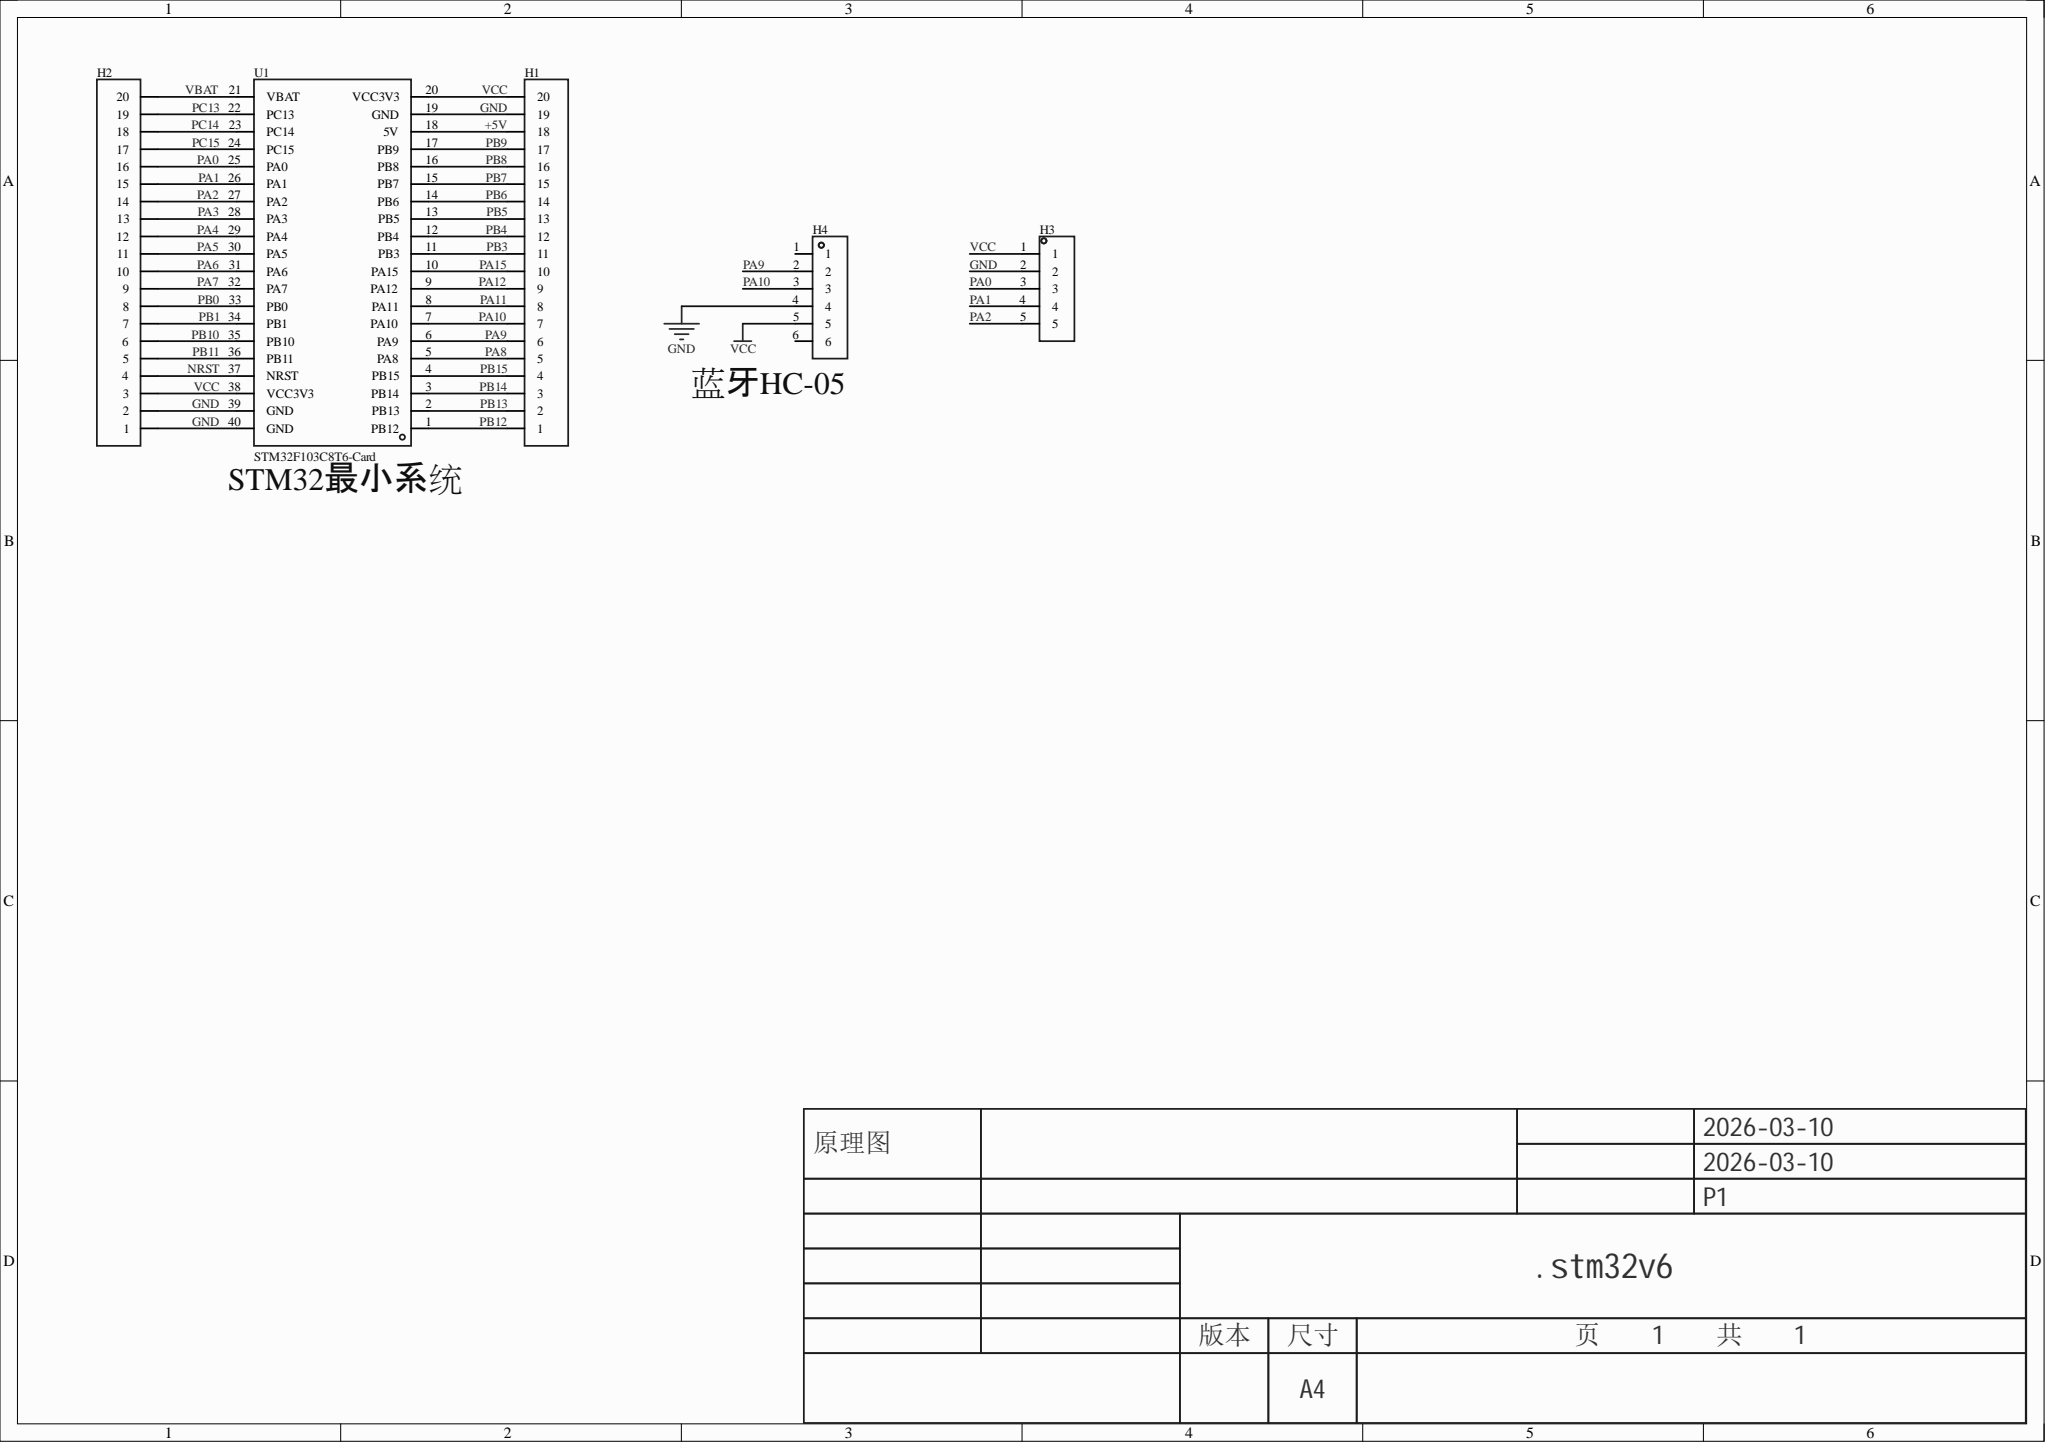Circuit board | Altium Designer | 5 parts | 37 nets
Bill of materials:
Comment,Description,Designator,Footprint,LibRef,Quantity
"","","H1, H2","HDR-TH_20P-P2.54-V-F","HDR-F_2.54_1x20P","2"
"","","H3","HDR-TH_5P-P2.54-V-M","HDR-M_2.54_1x5P","1"
"","","H4","HDR-TH_6P-P2.54-V-F","HDR-F_2.54_1x6P","1"
"STM32F103C8T6-Card","","U1","CONN-TH_L53.3-W22.9_STM32F103C8T6-CARD","STM32F103C8T6-Card","1"
Netlist (Protel format):
[
H1
HDR-TH_20P-P2.54-V-F




]
[
H2
HDR-TH_20P-P2.54-V-F




]
[
H3
HDR-TH_5P-P2.54-V-M




]
[
H4
HDR-TH_6P-P2.54-V-F




]
[
U1
CONN-TH_L53.3-W22.9_STM32F103C8T6-CARD
STM32F103C8T6-Card



]
(
VCC
H1-20
H2-3
H3-1
H4-5
U1-20
U1-38
)
(
VBAT
H2-20
U1-21
)
(
PC15
H2-17
U1-24
)
(
PC14
H2-18
U1-23
)
(
PC13
H2-19
U1-22
)
(
PB15
H1-4
U1-4
)
(
PB14
H1-3
U1-3
)
(
PB13
H1-2
U1-2
)
(
PB12
H1-1
U1-1
)
(
PB11
H2-5
U1-36
)
(
PB10
H2-6
U1-35
)
(
PB9
H1-17
U1-17
)
(
PB8
H1-16
U1-16
)
(
PB7
H1-15
U1-15
)
(
PB6
H1-14
U1-14
)
(
PB5
H1-13
U1-13
)
(
PB4
H1-12
U1-12
)
(
PB3
H1-11
U1-11
)
(
PB1
H2-7
U1-34
)
(
PB0
H2-8
U1-33
)
(
PA15
H1-10
U1-10
)
(
PA12
H1-9
U1-9
)
(
PA11
H1-8
U1-8
)
(
PA10
H1-7
H4-3
U1-7
)
(
PA9
H1-6
H4-2
U1-6
)
(
PA8
H1-5
U1-5
)
(
PA7
H2-9
U1-32
)
(
PA6
H2-10
U1-31
)
(
PA5
H2-11
U1-30
)
(
PA4
H2-12
U1-29
)
(
PA3
H2-13
U1-28
)
(
PA2
H2-14
H3-5
U1-27
)
(
PA1
H2-15
H3-4
U1-26
)
(
PA0
H2-16
H3-3
U1-25
)
(
NRST
H2-4
U1-37
)
(
GND
H1-19
H2-1
H2-2
H3-2
H4-4
U1-19
U1-39
U1-40
)
(
+5V
H1-18
U1-18
)